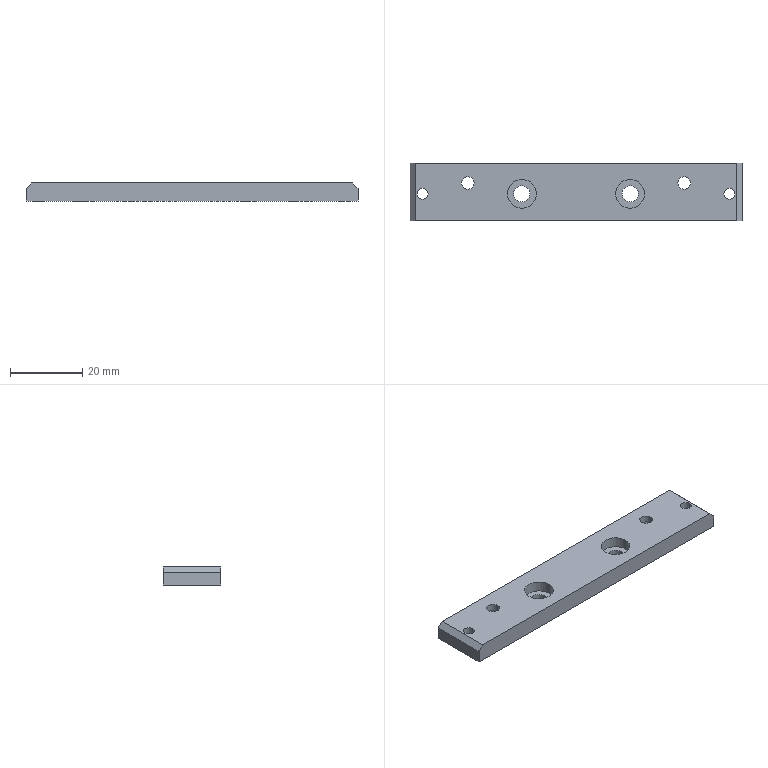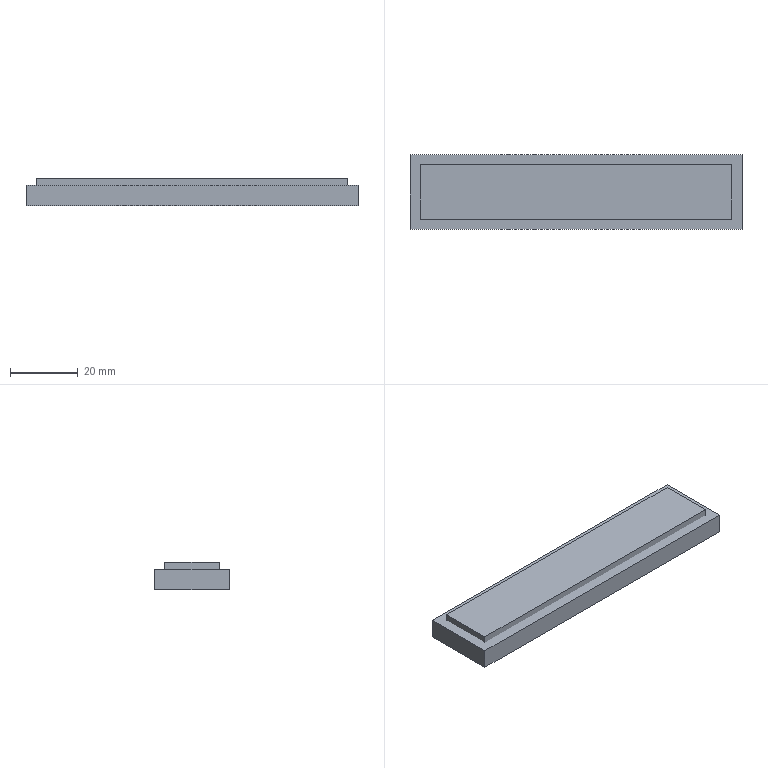CAM job | NX | 3-axis milling, drilling | part box 92 x 16 x 5 mm | stock box 98 x 22 x 8 mm
Tools:
number,name,description,diameter,corner_radius,flute_length,length,flutes
3,D63,Milling Tool-5 Parameters,63.0,0.0,50.0,75.0,2
1,D6A45,Milling Tool-5 Parameters,6.0,0.0,50.0,75.0,2
13,3.5ZT,Drilling Tool,3.5,0.0,35.0,50.0,2
12,4.5ZT,Drilling Tool,4.5,0.0,35.0,50.0,2
18,D2,Milling Tool-5 Parameters,2.0,0.0,50.0,75.0,2
16,D6,Milling Tool-5 Parameters,6.0,0.0,50.0,75.0,2
4,D10,Milling Tool-5 Parameters,10.0,0.0,50.0,75.0,2
14,D10JING,Milling Tool-5 Parameters,10.0,0.0,50.0,75.0,2
17,D4,Milling Tool-5 Parameters,4.0,0.0,50.0,75.0,2
Operations:
program,operation,operation_type,tool,method,geometry_group,spindle_rpm,surface_speed,feed_per_tooth,feed_cut,feed_plunge,cut_length_mm,path_length_mm,cut_time_min,machine_time_min
1,FLOOR_WALL,VolumeBased25DMillingOperation,D63,METHOD,A,6500.0,1286.0,0.1154,1500.0,100.0,173.0,227.0,0.1153,0.1207
1,DRILLING,Operation,D6A45,METHOD,A,5000.0,94.0,0.025,250.0,0.0,24.0,210.727,0.096,0.1147
1,DRILLING_COPY,Operation,3.5ZT,METHOD,A,2000.0,21.0,0.0375,150.0,0.0,15.103,153.281,0.1007,0.1145
1,DRILLING_COPY_COPY,Operation,4.5ZT,METHOD,A,2000.0,21.0,0.0375,150.0,0.0,21.704,136.557,0.1447,0.1562
1,HOLE_MILLING,CylinderMilling,D2,METHOD,A,7500.0,47.0,0.0667,1000.0,100.0,216.119,430.119,0.2161,0.2375
1,HOLE_MILLING_COPY,CylinderMilling,D6,METHOD,A,7500.0,141.0,0.1,1500.0,100.0,107.092,262.092,0.0714,0.0869
1,ADAPTIVE_MILLING,CavityMilling,D10,METHOD,A,7500.0,235.0,0.2,3000.0,1000.0,1235.82,1299.82,0.4139,0.4203
1,ZLEVEL_PROFILE,ZLevelMilling,D10JING,METHOD,A,7500.0,235.0,0.0667,1000.0,100.0,254.754,322.754,0.2548,0.2616
1,PLANAR_MILL,PlanarMilling,D6A45,METHOD,A,7500.0,141.0,0.0833,1250.0,100.0,301.558,864.093,0.2412,0.2975
1,PLANAR_MILL_COPY,PlanarMilling,D6A45,METHOD,A,7500.0,141.0,0.0833,1250.0,100.0,78.981,456.274,0.0632,0.1009
1,刀补18,CylinderMilling,D2,METHOD,A,7500.0,47.0,0.0667,1000.0,100.0,42.285,256.286,0.0423,0.0637
2,FLOOR_WALL_COPY,VolumeBased25DMillingOperation,D63,METHOD,B,6500.0,1286.0,0.1154,1500.0,100.0,501.0,979.001,0.334,0.3818
2,HOLE_MILLING_COPY_COPY,CylinderMilling,D4,METHOD,B,7500.0,141.0,0.1,1500.0,100.0,141.888,326.888,0.0946,0.1131
2,PLANAR_MILL_COPY_1,PlanarMilling,D6A45,METHOD,B,7500.0,141.0,0.0833,1250.0,100.0,298.277,868.951,0.2386,0.2957